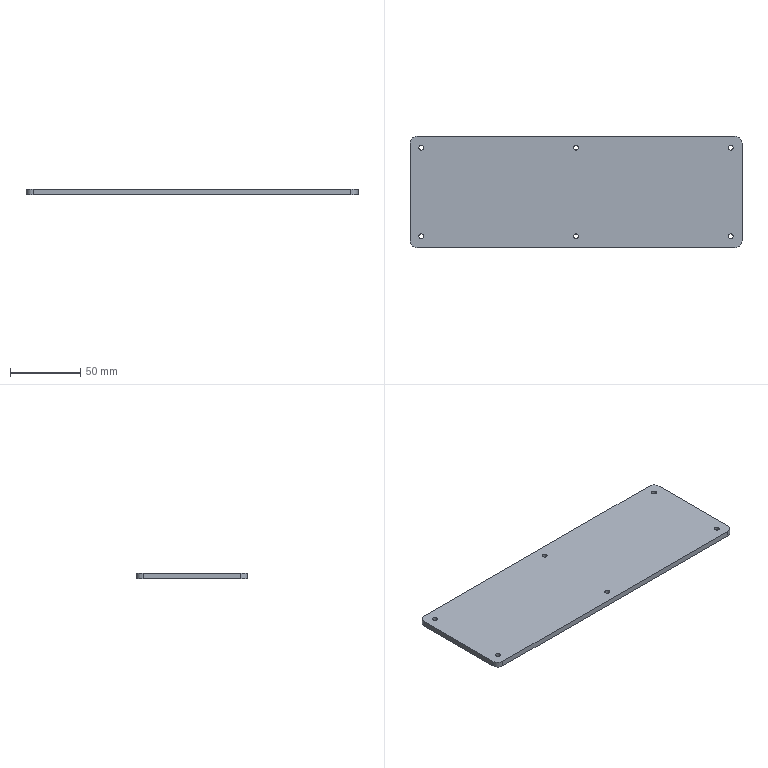Part | SolidWorks | features Extrusion 1, Fillet 1, ICE 1 | 1 solid | 22 faces | box 236 x 79 x 4 mm | volume 74259 mm3 | cylinder 16 | plane 6 | commonest cylinder face diameters 3.5 x12 10 x4
STEP:
#1=CARTESIAN_POINT('',(-108.25,31.5,4.));
#2=VERTEX_POINT('',#1);
#3=CARTESIAN_POINT('',(-111.75,31.5,4.));
#4=VERTEX_POINT('',#3);
#5=CARTESIAN_POINT('',(-110.,31.5,4.));
#6=DIRECTION('',(0.,0.,-1.));
#7=DIRECTION('',(-1.,0.,0.));
#8=AXIS2_PLACEMENT_3D('',#5,#6,#7);
#9=CIRCLE('',#8,1.75);
#10=EDGE_CURVE('',#2,#4,#9,.T.);
#11=ORIENTED_EDGE('',*,*,#10,.F.);
#12=CARTESIAN_POINT('',(-108.25,31.5,0.));
#13=VERTEX_POINT('',#12);
#14=CARTESIAN_POINT('',(-108.25,31.5,4.));
#15=DIRECTION('',(0.,0.,-1.));
#16=VECTOR('',#15,1000.);
#17=LINE('',#14,#16);
#18=EDGE_CURVE('',#2,#13,#17,.T.);
#19=ORIENTED_EDGE('',*,*,#18,.T.);
#20=CARTESIAN_POINT('',(-111.75,31.5,0.));
#21=VERTEX_POINT('',#20);
#22=CARTESIAN_POINT('',(-110.,31.5,0.));
#23=DIRECTION('',(0.,0.,-1.));
#24=DIRECTION('',(-1.,0.,0.));
#25=AXIS2_PLACEMENT_3D('',#22,#23,#24);
#26=CIRCLE('',#25,1.75);
#27=EDGE_CURVE('',#13,#21,#26,.T.);
#28=ORIENTED_EDGE('',*,*,#27,.T.);
#29=CARTESIAN_POINT('',(-111.75,31.5,4.));
#30=DIRECTION('',(0.,0.,-1.));
#31=VECTOR('',#30,1000.);
#32=LINE('',#29,#31);
#33=EDGE_CURVE('',#4,#21,#32,.T.);
#34=ORIENTED_EDGE('',*,*,#33,.F.);
#35=EDGE_LOOP('',(#11,#19,#28,#34));
#36=FACE_OUTER_BOUND('',#35,.T.);
#37=CARTESIAN_POINT('',(-110.,31.5,4.));
#38=DIRECTION('',(0.,0.,-1.));
#39=DIRECTION('',(-1.,0.,0.));
#40=AXIS2_PLACEMENT_3D('',#37,#38,#39);
#41=CYLINDRICAL_SURFACE('',#40,1.75);
#42=ADVANCED_FACE('',(#36),#41,.F.);
#43=CARTESIAN_POINT('',(-108.25,-31.5,4.));
#44=VERTEX_POINT('',#43);
#45=CARTESIAN_POINT('',(-111.75,-31.5,4.));
#46=VERTEX_POINT('',#45);
#47=CARTESIAN_POINT('',(-110.,-31.5,4.));
#48=DIRECTION('',(0.,0.,-1.));
#49=DIRECTION('',(-1.,0.,0.));
#50=AXIS2_PLACEMENT_3D('',#47,#48,#49);
#51=CIRCLE('',#50,1.75);
#52=EDGE_CURVE('',#44,#46,#51,.T.);
#53=ORIENTED_EDGE('',*,*,#52,.F.);
#54=CARTESIAN_POINT('',(-108.25,-31.5,0.));
#55=VERTEX_POINT('',#54);
#56=CARTESIAN_POINT('',(-108.25,-31.5,4.));
#57=DIRECTION('',(0.,0.,-1.));
#58=VECTOR('',#57,1000.);
#59=LINE('',#56,#58);
#60=EDGE_CURVE('',#44,#55,#59,.T.);
#61=ORIENTED_EDGE('',*,*,#60,.T.);
#62=CARTESIAN_POINT('',(-111.75,-31.5,0.));
#63=VERTEX_POINT('',#62);
#64=CARTESIAN_POINT('',(-110.,-31.5,0.));
#65=DIRECTION('',(0.,0.,-1.));
#66=DIRECTION('',(-1.,0.,0.));
#67=AXIS2_PLACEMENT_3D('',#64,#65,#66);
#68=CIRCLE('',#67,1.75);
#69=EDGE_CURVE('',#55,#63,#68,.T.);
#70=ORIENTED_EDGE('',*,*,#69,.T.);
#71=CARTESIAN_POINT('',(-111.75,-31.5,4.));
#72=DIRECTION('',(0.,0.,-1.));
#73=VECTOR('',#72,1000.);
#74=LINE('',#71,#73);
#75=EDGE_CURVE('',#46,#63,#74,.T.);
#76=ORIENTED_EDGE('',*,*,#75,.F.);
#77=EDGE_LOOP('',(#53,#61,#70,#76));
#78=FACE_OUTER_BOUND('',#77,.T.);
#79=CARTESIAN_POINT('',(-110.,-31.5,4.));
#80=DIRECTION('',(0.,0.,-1.));
#81=DIRECTION('',(-1.,0.,0.));
#82=AXIS2_PLACEMENT_3D('',#79,#80,#81);
#83=CYLINDRICAL_SURFACE('',#82,1.75);
#84=ADVANCED_FACE('',(#78),#83,.F.);
#85=CARTESIAN_POINT('',(111.75,-31.5,4.));
#86=VERTEX_POINT('',#85);
#87=CARTESIAN_POINT('',(108.25,-31.5,4.));
#88=VERTEX_POINT('',#87);
#89=CARTESIAN_POINT('',(110.,-31.5,4.));
#90=DIRECTION('',(0.,0.,-1.));
#91=DIRECTION('',(-1.,0.,0.));
#92=AXIS2_PLACEMENT_3D('',#89,#90,#91);
#93=CIRCLE('',#92,1.75);
#94=EDGE_CURVE('',#86,#88,#93,.T.);
#95=ORIENTED_EDGE('',*,*,#94,.F.);
#96=CARTESIAN_POINT('',(111.75,-31.5,0.));
#97=VERTEX_POINT('',#96);
#98=CARTESIAN_POINT('',(111.75,-31.5,4.));
#99=DIRECTION('',(0.,0.,-1.));
#100=VECTOR('',#99,1000.);
#101=LINE('',#98,#100);
#102=EDGE_CURVE('',#86,#97,#101,.T.);
#103=ORIENTED_EDGE('',*,*,#102,.T.);
#104=CARTESIAN_POINT('',(108.25,-31.5,0.));
#105=VERTEX_POINT('',#104);
#106=CARTESIAN_POINT('',(110.,-31.5,0.));
#107=DIRECTION('',(0.,0.,-1.));
#108=DIRECTION('',(-1.,0.,0.));
#109=AXIS2_PLACEMENT_3D('',#106,#107,#108);
#110=CIRCLE('',#109,1.75);
#111=EDGE_CURVE('',#97,#105,#110,.T.);
#112=ORIENTED_EDGE('',*,*,#111,.T.);
#113=CARTESIAN_POINT('',(108.25,-31.5,4.));
#114=DIRECTION('',(0.,0.,-1.));
#115=VECTOR('',#114,1000.);
#116=LINE('',#113,#115);
#117=EDGE_CURVE('',#88,#105,#116,.T.);
#118=ORIENTED_EDGE('',*,*,#117,.F.);
#119=EDGE_LOOP('',(#95,#103,#112,#118));
#120=FACE_OUTER_BOUND('',#119,.T.);
#121=CARTESIAN_POINT('',(110.,-31.5,4.));
#122=DIRECTION('',(0.,0.,-1.));
#123=DIRECTION('',(-1.,0.,0.));
#124=AXIS2_PLACEMENT_3D('',#121,#122,#123);
#125=CYLINDRICAL_SURFACE('',#124,1.75);
#126=ADVANCED_FACE('',(#120),#125,.F.);
#127=CARTESIAN_POINT('',(1.75,31.5,4.));
#128=VERTEX_POINT('',#127);
#129=CARTESIAN_POINT('',(-1.75,31.5,4.));
#130=VERTEX_POINT('',#129);
#131=CARTESIAN_POINT('',(0.,31.5,4.));
#132=DIRECTION('',(0.,0.,-1.));
#133=DIRECTION('',(-1.,0.,0.));
#134=AXIS2_PLACEMENT_3D('',#131,#132,#133);
#135=CIRCLE('',#134,1.75);
#136=EDGE_CURVE('',#128,#130,#135,.T.);
#137=ORIENTED_EDGE('',*,*,#136,.F.);
#138=CARTESIAN_POINT('',(1.75,31.5,0.));
#139=VERTEX_POINT('',#138);
#140=CARTESIAN_POINT('',(1.75,31.5,4.));
#141=DIRECTION('',(0.,0.,-1.));
#142=VECTOR('',#141,1000.);
#143=LINE('',#140,#142);
#144=EDGE_CURVE('',#128,#139,#143,.T.);
#145=ORIENTED_EDGE('',*,*,#144,.T.);
#146=CARTESIAN_POINT('',(-1.75,31.5,0.));
#147=VERTEX_POINT('',#146);
#148=CARTESIAN_POINT('',(0.,31.5,0.));
#149=DIRECTION('',(0.,0.,-1.));
#150=DIRECTION('',(-1.,0.,0.));
#151=AXIS2_PLACEMENT_3D('',#148,#149,#150);
#152=CIRCLE('',#151,1.75);
#153=EDGE_CURVE('',#139,#147,#152,.T.);
#154=ORIENTED_EDGE('',*,*,#153,.T.);
#155=CARTESIAN_POINT('',(-1.75,31.5,4.));
#156=DIRECTION('',(0.,0.,-1.));
#157=VECTOR('',#156,1000.);
#158=LINE('',#155,#157);
#159=EDGE_CURVE('',#130,#147,#158,.T.);
#160=ORIENTED_EDGE('',*,*,#159,.F.);
#161=EDGE_LOOP('',(#137,#145,#154,#160));
#162=FACE_OUTER_BOUND('',#161,.T.);
#163=CARTESIAN_POINT('',(0.,31.5,4.));
#164=DIRECTION('',(0.,0.,-1.));
#165=DIRECTION('',(-1.,0.,0.));
#166=AXIS2_PLACEMENT_3D('',#163,#164,#165);
#167=CYLINDRICAL_SURFACE('',#166,1.75);
#168=ADVANCED_FACE('',(#162),#167,.F.);
#169=CARTESIAN_POINT('',(1.75,-31.5,4.));
#170=VERTEX_POINT('',#169);
#171=CARTESIAN_POINT('',(-1.75,-31.5,4.));
#172=VERTEX_POINT('',#171);
#173=CARTESIAN_POINT('',(0.,-31.5,4.));
#174=DIRECTION('',(0.,0.,-1.));
#175=DIRECTION('',(-1.,0.,0.));
#176=AXIS2_PLACEMENT_3D('',#173,#174,#175);
#177=CIRCLE('',#176,1.75);
#178=EDGE_CURVE('',#170,#172,#177,.T.);
#179=ORIENTED_EDGE('',*,*,#178,.F.);
#180=CARTESIAN_POINT('',(1.75,-31.5,0.));
#181=VERTEX_POINT('',#180);
#182=CARTESIAN_POINT('',(1.75,-31.5,4.));
#183=DIRECTION('',(0.,0.,-1.));
#184=VECTOR('',#183,1000.);
#185=LINE('',#182,#184);
#186=EDGE_CURVE('',#170,#181,#185,.T.);
#187=ORIENTED_EDGE('',*,*,#186,.T.);
#188=CARTESIAN_POINT('',(-1.75,-31.5,0.));
#189=VERTEX_POINT('',#188);
#190=CARTESIAN_POINT('',(0.,-31.5,0.));
#191=DIRECTION('',(0.,0.,-1.));
#192=DIRECTION('',(-1.,0.,0.));
#193=AXIS2_PLACEMENT_3D('',#190,#191,#192);
#194=CIRCLE('',#193,1.75);
#195=EDGE_CURVE('',#181,#189,#194,.T.);
#196=ORIENTED_EDGE('',*,*,#195,.T.);
#197=CARTESIAN_POINT('',(-1.75,-31.5,4.));
#198=DIRECTION('',(0.,0.,-1.));
#199=VECTOR('',#198,1000.);
#200=LINE('',#197,#199);
#201=EDGE_CURVE('',#172,#189,#200,.T.);
#202=ORIENTED_EDGE('',*,*,#201,.F.);
#203=EDGE_LOOP('',(#179,#187,#196,#202));
#204=FACE_OUTER_BOUND('',#203,.T.);
#205=CARTESIAN_POINT('',(0.,-31.5,4.));
#206=DIRECTION('',(0.,0.,-1.));
#207=DIRECTION('',(-1.,0.,0.));
#208=AXIS2_PLACEMENT_3D('',#205,#206,#207);
#209=CYLINDRICAL_SURFACE('',#208,1.75);
#210=ADVANCED_FACE('',(#204),#209,.F.);
#211=CARTESIAN_POINT('',(111.75,31.5,4.));
#212=VERTEX_POINT('',#211);
#213=CARTESIAN_POINT('',(108.25,31.5,4.));
#214=VERTEX_POINT('',#213);
#215=CARTESIAN_POINT('',(110.,31.5,4.));
#216=DIRECTION('',(0.,0.,-1.));
#217=DIRECTION('',(-1.,0.,0.));
#218=AXIS2_PLACEMENT_3D('',#215,#216,#217);
#219=CIRCLE('',#218,1.75);
#220=EDGE_CURVE('',#212,#214,#219,.T.);
#221=ORIENTED_EDGE('',*,*,#220,.F.);
#222=CARTESIAN_POINT('',(111.75,31.5,0.));
#223=VERTEX_POINT('',#222);
#224=CARTESIAN_POINT('',(111.75,31.5,4.));
#225=DIRECTION('',(0.,0.,-1.));
#226=VECTOR('',#225,1000.);
#227=LINE('',#224,#226);
#228=EDGE_CURVE('',#212,#223,#227,.T.);
#229=ORIENTED_EDGE('',*,*,#228,.T.);
#230=CARTESIAN_POINT('',(108.25,31.5,0.));
#231=VERTEX_POINT('',#230);
#232=CARTESIAN_POINT('',(110.,31.5,0.));
#233=DIRECTION('',(0.,0.,-1.));
#234=DIRECTION('',(-1.,0.,0.));
#235=AXIS2_PLACEMENT_3D('',#232,#233,#234);
#236=CIRCLE('',#235,1.75);
#237=EDGE_CURVE('',#223,#231,#236,.T.);
#238=ORIENTED_EDGE('',*,*,#237,.T.);
#239=CARTESIAN_POINT('',(108.25,31.5,4.));
#240=DIRECTION('',(0.,0.,-1.));
#241=VECTOR('',#240,1000.);
#242=LINE('',#239,#241);
#243=EDGE_CURVE('',#214,#231,#242,.T.);
#244=ORIENTED_EDGE('',*,*,#243,.F.);
#245=EDGE_LOOP('',(#221,#229,#238,#244));
#246=FACE_OUTER_BOUND('',#245,.T.);
#247=CARTESIAN_POINT('',(110.,31.5,4.));
#248=DIRECTION('',(0.,0.,-1.));
#249=DIRECTION('',(-1.,0.,0.));
#250=AXIS2_PLACEMENT_3D('',#247,#248,#249);
#251=CYLINDRICAL_SURFACE('',#250,1.75);
#252=ADVANCED_FACE('',(#246),#251,.F.);
#253=CARTESIAN_POINT('',(-118.,34.5,0.));
#254=VERTEX_POINT('',#253);
#255=CARTESIAN_POINT('',(-118.,-34.5,0.));
#256=VERTEX_POINT('',#255);
#257=CARTESIAN_POINT('',(-118.,-39.5,0.));
#258=DIRECTION('',(0.,-1.,0.));
#259=VECTOR('',#258,1000.);
#260=LINE('',#257,#259);
#261=EDGE_CURVE('',#254,#256,#260,.T.);
#262=ORIENTED_EDGE('',*,*,#261,.T.);
#263=CARTESIAN_POINT('',(-118.,-34.5,4.));
#264=VERTEX_POINT('',#263);
#265=CARTESIAN_POINT('',(-118.,-34.5,4.));
#266=DIRECTION('',(0.,0.,1.));
#267=VECTOR('',#266,1000.);
#268=LINE('',#265,#267);
#269=EDGE_CURVE('',#256,#264,#268,.T.);
#270=ORIENTED_EDGE('',*,*,#269,.T.);
#271=CARTESIAN_POINT('',(-118.,34.5,4.));
#272=VERTEX_POINT('',#271);
#273=CARTESIAN_POINT('',(-118.,-39.5,4.));
#274=DIRECTION('',(0.,-1.,0.));
#275=VECTOR('',#274,1000.);
#276=LINE('',#273,#275);
#277=EDGE_CURVE('',#272,#264,#276,.T.);
#278=ORIENTED_EDGE('',*,*,#277,.F.);
#279=CARTESIAN_POINT('',(-118.,34.5,4.));
#280=DIRECTION('',(0.,0.,-1.));
#281=VECTOR('',#280,1000.);
#282=LINE('',#279,#281);
#283=EDGE_CURVE('',#272,#254,#282,.T.);
#284=ORIENTED_EDGE('',*,*,#283,.T.);
#285=EDGE_LOOP('',(#262,#270,#278,#284));
#286=FACE_OUTER_BOUND('',#285,.T.);
#287=CARTESIAN_POINT('',(-118.,-39.5,4.));
#288=DIRECTION('',(1.,0.,0.));
#289=DIRECTION('',(0.,0.,-1.));
#290=AXIS2_PLACEMENT_3D('',#287,#288,#289);
#291=PLANE('',#290);
#292=ADVANCED_FACE('',(#286),#291,.F.);
#293=CARTESIAN_POINT('',(-113.,-39.5,0.));
#294=VERTEX_POINT('',#293);
#295=CARTESIAN_POINT('',(113.,-39.5,0.));
#296=VERTEX_POINT('',#295);
#297=CARTESIAN_POINT('',(118.,-39.5,0.));
#298=DIRECTION('',(1.,0.,0.));
#299=VECTOR('',#298,1000.);
#300=LINE('',#297,#299);
#301=EDGE_CURVE('',#294,#296,#300,.T.);
#302=ORIENTED_EDGE('',*,*,#301,.T.);
#303=CARTESIAN_POINT('',(113.,-39.5,4.));
#304=VERTEX_POINT('',#303);
#305=CARTESIAN_POINT('',(113.,-39.5,4.));
#306=DIRECTION('',(0.,0.,1.));
#307=VECTOR('',#306,1000.);
#308=LINE('',#305,#307);
#309=EDGE_CURVE('',#296,#304,#308,.T.);
#310=ORIENTED_EDGE('',*,*,#309,.T.);
#311=CARTESIAN_POINT('',(-113.,-39.5,4.));
#312=VERTEX_POINT('',#311);
#313=CARTESIAN_POINT('',(118.,-39.5,4.));
#314=DIRECTION('',(1.,0.,0.));
#315=VECTOR('',#314,1000.);
#316=LINE('',#313,#315);
#317=EDGE_CURVE('',#312,#304,#316,.T.);
#318=ORIENTED_EDGE('',*,*,#317,.F.);
#319=CARTESIAN_POINT('',(-113.,-39.5,4.));
#320=DIRECTION('',(0.,0.,-1.));
#321=VECTOR('',#320,1000.);
#322=LINE('',#319,#321);
#323=EDGE_CURVE('',#312,#294,#322,.T.);
#324=ORIENTED_EDGE('',*,*,#323,.T.);
#325=EDGE_LOOP('',(#302,#310,#318,#324));
#326=FACE_OUTER_BOUND('',#325,.T.);
#327=CARTESIAN_POINT('',(118.,-39.5,4.));
#328=DIRECTION('',(0.,1.,0.));
#329=DIRECTION('',(-1.,0.,0.));
#330=AXIS2_PLACEMENT_3D('',#327,#328,#329);
#331=PLANE('',#330);
#332=ADVANCED_FACE('',(#326),#331,.F.);
#333=CARTESIAN_POINT('',(118.,-34.5,0.));
#334=VERTEX_POINT('',#333);
#335=CARTESIAN_POINT('',(118.,34.5,0.));
#336=VERTEX_POINT('',#335);
#337=CARTESIAN_POINT('',(118.,-39.5,0.));
#338=DIRECTION('',(0.,1.,0.));
#339=VECTOR('',#338,1000.);
#340=LINE('',#337,#339);
#341=EDGE_CURVE('',#334,#336,#340,.T.);
#342=ORIENTED_EDGE('',*,*,#341,.T.);
#343=CARTESIAN_POINT('',(118.,34.5,4.));
#344=VERTEX_POINT('',#343);
#345=CARTESIAN_POINT('',(118.,34.5,4.));
#346=DIRECTION('',(0.,0.,1.));
#347=VECTOR('',#346,1000.);
#348=LINE('',#345,#347);
#349=EDGE_CURVE('',#336,#344,#348,.T.);
#350=ORIENTED_EDGE('',*,*,#349,.T.);
#351=CARTESIAN_POINT('',(118.,-34.5,4.));
#352=VERTEX_POINT('',#351);
#353=CARTESIAN_POINT('',(118.,-39.5,4.));
#354=DIRECTION('',(0.,1.,0.));
#355=VECTOR('',#354,1000.);
#356=LINE('',#353,#355);
#357=EDGE_CURVE('',#352,#344,#356,.T.);
#358=ORIENTED_EDGE('',*,*,#357,.F.);
#359=CARTESIAN_POINT('',(118.,-34.5,4.));
#360=DIRECTION('',(0.,0.,-1.));
#361=VECTOR('',#360,1000.);
#362=LINE('',#359,#361);
#363=EDGE_CURVE('',#352,#334,#362,.T.);
#364=ORIENTED_EDGE('',*,*,#363,.T.);
#365=EDGE_LOOP('',(#342,#350,#358,#364));
#366=FACE_OUTER_BOUND('',#365,.T.);
#367=CARTESIAN_POINT('',(118.,-39.5,4.));
#368=DIRECTION('',(-1.,0.,0.));
#369=DIRECTION('',(0.,0.,1.));
#370=AXIS2_PLACEMENT_3D('',#367,#368,#369);
#371=PLANE('',#370);
#372=ADVANCED_FACE('',(#366),#371,.F.);
#373=CARTESIAN_POINT('',(113.,39.5,4.));
#374=VERTEX_POINT('',#373);
#375=CARTESIAN_POINT('',(-113.,39.5,4.));
#376=VERTEX_POINT('',#375);
#377=CARTESIAN_POINT('',(118.,39.5,4.));
#378=DIRECTION('',(-1.,0.,0.));
#379=VECTOR('',#378,1000.);
#380=LINE('',#377,#379);
#381=EDGE_CURVE('',#374,#376,#380,.T.);
#382=ORIENTED_EDGE('',*,*,#381,.F.);
#383=CARTESIAN_POINT('',(113.,39.5,0.));
#384=VERTEX_POINT('',#383);
#385=CARTESIAN_POINT('',(113.,39.5,4.));
#386=DIRECTION('',(0.,0.,-1.));
#387=VECTOR('',#386,1000.);
#388=LINE('',#385,#387);
#389=EDGE_CURVE('',#374,#384,#388,.T.);
#390=ORIENTED_EDGE('',*,*,#389,.T.);
#391=CARTESIAN_POINT('',(-113.,39.5,0.));
#392=VERTEX_POINT('',#391);
#393=CARTESIAN_POINT('',(118.,39.5,0.));
#394=DIRECTION('',(-1.,0.,0.));
#395=VECTOR('',#394,1000.);
#396=LINE('',#393,#395);
#397=EDGE_CURVE('',#384,#392,#396,.T.);
#398=ORIENTED_EDGE('',*,*,#397,.T.);
#399=CARTESIAN_POINT('',(-113.,39.5,4.));
#400=DIRECTION('',(0.,0.,1.));
#401=VECTOR('',#400,1000.);
#402=LINE('',#399,#401);
#403=EDGE_CURVE('',#392,#376,#402,.T.);
#404=ORIENTED_EDGE('',*,*,#403,.T.);
#405=EDGE_LOOP('',(#382,#390,#398,#404));
#406=FACE_OUTER_BOUND('',#405,.T.);
#407=CARTESIAN_POINT('',(118.,39.5,4.));
#408=DIRECTION('',(0.,-1.,0.));
#409=DIRECTION('',(1.,0.,0.));
#410=AXIS2_PLACEMENT_3D('',#407,#408,#409);
#411=PLANE('',#410);
#412=ADVANCED_FACE('',(#406),#411,.F.);
#413=CARTESIAN_POINT('',(-110.,31.5,4.));
#414=DIRECTION('',(0.,0.,-1.));
#415=DIRECTION('',(-1.,0.,0.));
#416=AXIS2_PLACEMENT_3D('',#413,#414,#415);
#417=CIRCLE('',#416,1.75);
#418=EDGE_CURVE('',#4,#2,#417,.T.);
#419=ORIENTED_EDGE('',*,*,#418,.T.);
#420=ORIENTED_EDGE('',*,*,#10,.T.);
#421=EDGE_LOOP('',(#419,#420));
#422=FACE_BOUND('',#421,.T.);
#423=CARTESIAN_POINT('',(-110.,-31.5,4.));
#424=DIRECTION('',(0.,0.,-1.));
#425=DIRECTION('',(-1.,0.,0.));
#426=AXIS2_PLACEMENT_3D('',#423,#424,#425);
#427=CIRCLE('',#426,1.75);
#428=EDGE_CURVE('',#46,#44,#427,.T.);
#429=ORIENTED_EDGE('',*,*,#428,.T.);
#430=ORIENTED_EDGE('',*,*,#52,.T.);
#431=EDGE_LOOP('',(#429,#430));
#432=FACE_BOUND('',#431,.T.);
#433=CARTESIAN_POINT('',(110.,-31.5,4.));
#434=DIRECTION('',(0.,0.,-1.));
#435=DIRECTION('',(-1.,0.,0.));
#436=AXIS2_PLACEMENT_3D('',#433,#434,#435);
#437=CIRCLE('',#436,1.75);
#438=EDGE_CURVE('',#88,#86,#437,.T.);
#439=ORIENTED_EDGE('',*,*,#438,.T.);
#440=ORIENTED_EDGE('',*,*,#94,.T.);
#441=EDGE_LOOP('',(#439,#440));
#442=FACE_BOUND('',#441,.T.);
#443=CARTESIAN_POINT('',(0.,31.5,4.));
#444=DIRECTION('',(0.,0.,-1.));
#445=DIRECTION('',(-1.,0.,0.));
#446=AXIS2_PLACEMENT_3D('',#443,#444,#445);
#447=CIRCLE('',#446,1.75);
#448=EDGE_CURVE('',#130,#128,#447,.T.);
#449=ORIENTED_EDGE('',*,*,#448,.T.);
#450=ORIENTED_EDGE('',*,*,#136,.T.);
#451=EDGE_LOOP('',(#449,#450));
#452=FACE_BOUND('',#451,.T.);
#453=CARTESIAN_POINT('',(0.,-31.5,4.));
#454=DIRECTION('',(0.,0.,-1.));
#455=DIRECTION('',(-1.,0.,0.));
#456=AXIS2_PLACEMENT_3D('',#453,#454,#455);
#457=CIRCLE('',#456,1.75);
#458=EDGE_CURVE('',#172,#170,#457,.T.);
#459=ORIENTED_EDGE('',*,*,#458,.T.);
#460=ORIENTED_EDGE('',*,*,#178,.T.);
#461=EDGE_LOOP('',(#459,#460));
#462=FACE_BOUND('',#461,.T.);
#463=CARTESIAN_POINT('',(110.,31.5,4.));
#464=DIRECTION('',(0.,0.,-1.));
#465=DIRECTION('',(-1.,0.,0.));
#466=AXIS2_PLACEMENT_3D('',#463,#464,#465);
#467=CIRCLE('',#466,1.75);
#468=EDGE_CURVE('',#214,#212,#467,.T.);
#469=ORIENTED_EDGE('',*,*,#468,.T.);
#470=ORIENTED_EDGE('',*,*,#220,.T.);
#471=EDGE_LOOP('',(#469,#470));
#472=FACE_BOUND('',#471,.T.);
#473=ORIENTED_EDGE('',*,*,#357,.T.);
#474=CARTESIAN_POINT('',(113.,34.5,4.));
#475=DIRECTION('',(0.,0.,1.));
#476=DIRECTION('',(1.,0.,0.));
#477=AXIS2_PLACEMENT_3D('',#474,#475,#476);
#478=CIRCLE('',#477,5.);
#479=EDGE_CURVE('',#344,#374,#478,.T.);
#480=ORIENTED_EDGE('',*,*,#479,.T.);
#481=ORIENTED_EDGE('',*,*,#381,.T.);
#482=CARTESIAN_POINT('',(-113.,34.5,4.));
#483=DIRECTION('',(0.,0.,1.));
#484=DIRECTION('',(1.,0.,0.));
#485=AXIS2_PLACEMENT_3D('',#482,#483,#484);
#486=CIRCLE('',#485,5.);
#487=EDGE_CURVE('',#376,#272,#486,.T.);
#488=ORIENTED_EDGE('',*,*,#487,.T.);
#489=ORIENTED_EDGE('',*,*,#277,.T.);
#490=CARTESIAN_POINT('',(-113.,-34.5,4.));
#491=DIRECTION('',(0.,0.,1.));
#492=DIRECTION('',(1.,0.,0.));
#493=AXIS2_PLACEMENT_3D('',#490,#491,#492);
#494=CIRCLE('',#493,5.);
#495=EDGE_CURVE('',#264,#312,#494,.T.);
#496=ORIENTED_EDGE('',*,*,#495,.T.);
#497=ORIENTED_EDGE('',*,*,#317,.T.);
#498=CARTESIAN_POINT('',(113.,-34.5,4.));
#499=DIRECTION('',(0.,0.,1.));
#500=DIRECTION('',(1.,0.,0.));
#501=AXIS2_PLACEMENT_3D('',#498,#499,#500);
#502=CIRCLE('',#501,5.);
#503=EDGE_CURVE('',#304,#352,#502,.T.);
#504=ORIENTED_EDGE('',*,*,#503,.T.);
#505=EDGE_LOOP('',(#473,#480,#481,#488,#489,#496,#497,#504));
#506=FACE_OUTER_BOUND('',#505,.T.);
#507=CARTESIAN_POINT('',(0.,0.,4.));
#508=DIRECTION('',(0.,0.,1.));
#509=DIRECTION('',(1.,0.,0.));
#510=AXIS2_PLACEMENT_3D('',#507,#508,#509);
#511=PLANE('',#510);
#512=ADVANCED_FACE('',(#422,#432,#442,#452,#462,#472,#506),#511,.T.);
#513=CARTESIAN_POINT('',(-110.,31.5,0.));
#514=DIRECTION('',(0.,0.,-1.));
#515=DIRECTION('',(-1.,0.,0.));
#516=AXIS2_PLACEMENT_3D('',#513,#514,#515);
#517=CIRCLE('',#516,1.75);
#518=EDGE_CURVE('',#21,#13,#517,.T.);
#519=ORIENTED_EDGE('',*,*,#518,.F.);
#520=ORIENTED_EDGE('',*,*,#27,.F.);
#521=EDGE_LOOP('',(#519,#520));
#522=FACE_BOUND('',#521,.T.);
#523=CARTESIAN_POINT('',(-110.,-31.5,0.));
#524=DIRECTION('',(0.,0.,-1.));
#525=DIRECTION('',(-1.,0.,0.));
#526=AXIS2_PLACEMENT_3D('',#523,#524,#525);
#527=CIRCLE('',#526,1.75);
#528=EDGE_CURVE('',#63,#55,#527,.T.);
#529=ORIENTED_EDGE('',*,*,#528,.F.);
#530=ORIENTED_EDGE('',*,*,#69,.F.);
#531=EDGE_LOOP('',(#529,#530));
#532=FACE_BOUND('',#531,.T.);
#533=CARTESIAN_POINT('',(110.,-31.5,0.));
#534=DIRECTION('',(0.,0.,-1.));
#535=DIRECTION('',(-1.,0.,0.));
#536=AXIS2_PLACEMENT_3D('',#533,#534,#535);
#537=CIRCLE('',#536,1.75);
#538=EDGE_CURVE('',#105,#97,#537,.T.);
#539=ORIENTED_EDGE('',*,*,#538,.F.);
#540=ORIENTED_EDGE('',*,*,#111,.F.);
#541=EDGE_LOOP('',(#539,#540));
#542=FACE_BOUND('',#541,.T.);
#543=CARTESIAN_POINT('',(0.,31.5,0.));
#544=DIRECTION('',(0.,0.,-1.));
#545=DIRECTION('',(-1.,0.,0.));
#546=AXIS2_PLACEMENT_3D('',#543,#544,#545);
#547=CIRCLE('',#546,1.75);
#548=EDGE_CURVE('',#147,#139,#547,.T.);
#549=ORIENTED_EDGE('',*,*,#548,.F.);
#550=ORIENTED_EDGE('',*,*,#153,.F.);
#551=EDGE_LOOP('',(#549,#550));
#552=FACE_BOUND('',#551,.T.);
#553=CARTESIAN_POINT('',(0.,-31.5,0.));
#554=DIRECTION('',(0.,0.,-1.));
#555=DIRECTION('',(-1.,0.,0.));
#556=AXIS2_PLACEMENT_3D('',#553,#554,#555);
#557=CIRCLE('',#556,1.75);
#558=EDGE_CURVE('',#189,#181,#557,.T.);
#559=ORIENTED_EDGE('',*,*,#558,.F.);
#560=ORIENTED_EDGE('',*,*,#195,.F.);
#561=EDGE_LOOP('',(#559,#560));
#562=FACE_BOUND('',#561,.T.);
#563=CARTESIAN_POINT('',(110.,31.5,0.));
#564=DIRECTION('',(0.,0.,-1.));
#565=DIRECTION('',(-1.,0.,0.));
#566=AXIS2_PLACEMENT_3D('',#563,#564,#565);
#567=CIRCLE('',#566,1.75);
#568=EDGE_CURVE('',#231,#223,#567,.T.);
#569=ORIENTED_EDGE('',*,*,#568,.F.);
#570=ORIENTED_EDGE('',*,*,#237,.F.);
#571=EDGE_LOOP('',(#569,#570));
#572=FACE_BOUND('',#571,.T.);
#573=ORIENTED_EDGE('',*,*,#397,.F.);
#574=CARTESIAN_POINT('',(113.,34.5,0.));
#575=DIRECTION('',(0.,0.,-1.));
#576=DIRECTION('',(1.,0.,0.));
#577=AXIS2_PLACEMENT_3D('',#574,#575,#576);
#578=CIRCLE('',#577,5.);
#579=EDGE_CURVE('',#384,#336,#578,.T.);
#580=ORIENTED_EDGE('',*,*,#579,.T.);
#581=ORIENTED_EDGE('',*,*,#341,.F.);
#582=CARTESIAN_POINT('',(113.,-34.5,0.));
#583=DIRECTION('',(0.,0.,-1.));
#584=DIRECTION('',(1.,0.,0.));
#585=AXIS2_PLACEMENT_3D('',#582,#583,#584);
#586=CIRCLE('',#585,5.);
#587=EDGE_CURVE('',#334,#296,#586,.T.);
#588=ORIENTED_EDGE('',*,*,#587,.T.);
#589=ORIENTED_EDGE('',*,*,#301,.F.);
#590=CARTESIAN_POINT('',(-113.,-34.5,0.));
#591=DIRECTION('',(0.,0.,-1.));
#592=DIRECTION('',(1.,0.,0.));
#593=AXIS2_PLACEMENT_3D('',#590,#591,#592);
#594=CIRCLE('',#593,5.);
#595=EDGE_CURVE('',#294,#256,#594,.T.);
#596=ORIENTED_EDGE('',*,*,#595,.T.);
#597=ORIENTED_EDGE('',*,*,#261,.F.);
#598=CARTESIAN_POINT('',(-113.,34.5,0.));
#599=DIRECTION('',(0.,0.,-1.));
#600=DIRECTION('',(1.,0.,0.));
#601=AXIS2_PLACEMENT_3D('',#598,#599,#600);
#602=CIRCLE('',#601,5.);
#603=EDGE_CURVE('',#254,#392,#602,.T.);
#604=ORIENTED_EDGE('',*,*,#603,.T.);
#605=EDGE_LOOP('',(#573,#580,#581,#588,#589,#596,#597,#604));
#606=FACE_OUTER_BOUND('',#605,.T.);
#607=CARTESIAN_POINT('',(0.,0.,0.));
#608=DIRECTION('',(0.,0.,1.));
#609=DIRECTION('',(1.,0.,0.));
#610=AXIS2_PLACEMENT_3D('',#607,#608,#609);
#611=PLANE('',#610);
#612=ADVANCED_FACE('',(#522,#532,#542,#552,#562,#572,#606),#611,.F.);
#613=ORIENTED_EDGE('',*,*,#479,.F.);
#614=ORIENTED_EDGE('',*,*,#349,.F.);
#615=ORIENTED_EDGE('',*,*,#579,.F.);
#616=ORIENTED_EDGE('',*,*,#389,.F.);
#617=EDGE_LOOP('',(#613,#614,#615,#616));
#618=FACE_OUTER_BOUND('',#617,.T.);
#619=CARTESIAN_POINT('',(113.,34.5,4.));
#620=DIRECTION('',(0.,0.,-1.));
#621=DIRECTION('',(-1.,0.,0.));
#622=AXIS2_PLACEMENT_3D('',#619,#620,#621);
#623=CYLINDRICAL_SURFACE('',#622,5.);
#624=ADVANCED_FACE('',(#618),#623,.T.);
#625=ORIENTED_EDGE('',*,*,#503,.F.);
#626=ORIENTED_EDGE('',*,*,#309,.F.);
#627=ORIENTED_EDGE('',*,*,#587,.F.);
#628=ORIENTED_EDGE('',*,*,#363,.F.);
#629=EDGE_LOOP('',(#625,#626,#627,#628));
#630=FACE_OUTER_BOUND('',#629,.T.);
#631=CARTESIAN_POINT('',(113.,-34.5,4.));
#632=DIRECTION('',(0.,0.,-1.));
#633=DIRECTION('',(-1.,0.,0.));
#634=AXIS2_PLACEMENT_3D('',#631,#632,#633);
#635=CYLINDRICAL_SURFACE('',#634,5.);
#636=ADVANCED_FACE('',(#630),#635,.T.);
#637=ORIENTED_EDGE('',*,*,#495,.F.);
#638=ORIENTED_EDGE('',*,*,#269,.F.);
#639=ORIENTED_EDGE('',*,*,#595,.F.);
#640=ORIENTED_EDGE('',*,*,#323,.F.);
#641=EDGE_LOOP('',(#637,#638,#639,#640));
#642=FACE_OUTER_BOUND('',#641,.T.);
#643=CARTESIAN_POINT('',(-113.,-34.5,4.));
#644=DIRECTION('',(0.,0.,-1.));
#645=DIRECTION('',(-1.,0.,0.));
#646=AXIS2_PLACEMENT_3D('',#643,#644,#645);
#647=CYLINDRICAL_SURFACE('',#646,5.);
#648=ADVANCED_FACE('',(#642),#647,.T.);
#649=ORIENTED_EDGE('',*,*,#487,.F.);
#650=ORIENTED_EDGE('',*,*,#403,.F.);
#651=ORIENTED_EDGE('',*,*,#603,.F.);
#652=ORIENTED_EDGE('',*,*,#283,.F.);
#653=EDGE_LOOP('',(#649,#650,#651,#652));
#654=FACE_OUTER_BOUND('',#653,.T.);
#655=CARTESIAN_POINT('',(-113.,34.5,4.));
#656=DIRECTION('',(0.,0.,-1.));
#657=DIRECTION('',(-1.,0.,0.));
#658=AXIS2_PLACEMENT_3D('',#655,#656,#657);
#659=CYLINDRICAL_SURFACE('',#658,5.);
#660=ADVANCED_FACE('',(#654),#659,.T.);
#661=ORIENTED_EDGE('',*,*,#228,.F.);
#662=ORIENTED_EDGE('',*,*,#468,.F.);
#663=ORIENTED_EDGE('',*,*,#243,.T.);
#664=ORIENTED_EDGE('',*,*,#568,.T.);
#665=EDGE_LOOP('',(#661,#662,#663,#664));
#666=FACE_OUTER_BOUND('',#665,.T.);
#667=CARTESIAN_POINT('',(110.,31.5,4.));
#668=DIRECTION('',(0.,0.,-1.));
#669=DIRECTION('',(-1.,0.,0.));
#670=AXIS2_PLACEMENT_3D('',#667,#668,#669);
#671=CYLINDRICAL_SURFACE('',#670,1.75);
#672=ADVANCED_FACE('',(#666),#671,.F.);
#673=ORIENTED_EDGE('',*,*,#186,.F.);
#674=ORIENTED_EDGE('',*,*,#458,.F.);
#675=ORIENTED_EDGE('',*,*,#201,.T.);
#676=ORIENTED_EDGE('',*,*,#558,.T.);
#677=EDGE_LOOP('',(#673,#674,#675,#676));
#678=FACE_OUTER_BOUND('',#677,.T.);
#679=CARTESIAN_POINT('',(0.,-31.5,4.));
#680=DIRECTION('',(0.,0.,-1.));
#681=DIRECTION('',(-1.,0.,0.));
#682=AXIS2_PLACEMENT_3D('',#679,#680,#681);
#683=CYLINDRICAL_SURFACE('',#682,1.75);
#684=ADVANCED_FACE('',(#678),#683,.F.);
#685=ORIENTED_EDGE('',*,*,#144,.F.);
#686=ORIENTED_EDGE('',*,*,#448,.F.);
#687=ORIENTED_EDGE('',*,*,#159,.T.);
#688=ORIENTED_EDGE('',*,*,#548,.T.);
#689=EDGE_LOOP('',(#685,#686,#687,#688));
#690=FACE_OUTER_BOUND('',#689,.T.);
#691=CARTESIAN_POINT('',(0.,31.5,4.));
#692=DIRECTION('',(0.,0.,-1.));
#693=DIRECTION('',(-1.,0.,0.));
#694=AXIS2_PLACEMENT_3D('',#691,#692,#693);
#695=CYLINDRICAL_SURFACE('',#694,1.75);
#696=ADVANCED_FACE('',(#690),#695,.F.);
#697=ORIENTED_EDGE('',*,*,#102,.F.);
#698=ORIENTED_EDGE('',*,*,#438,.F.);
#699=ORIENTED_EDGE('',*,*,#117,.T.);
#700=ORIENTED_EDGE('',*,*,#538,.T.);
#701=EDGE_LOOP('',(#697,#698,#699,#700));
#702=FACE_OUTER_BOUND('',#701,.T.);
#703=CARTESIAN_POINT('',(110.,-31.5,4.));
#704=DIRECTION('',(0.,0.,-1.));
#705=DIRECTION('',(-1.,0.,0.));
#706=AXIS2_PLACEMENT_3D('',#703,#704,#705);
#707=CYLINDRICAL_SURFACE('',#706,1.75);
#708=ADVANCED_FACE('',(#702),#707,.F.);
#709=ORIENTED_EDGE('',*,*,#60,.F.);
#710=ORIENTED_EDGE('',*,*,#428,.F.);
#711=ORIENTED_EDGE('',*,*,#75,.T.);
#712=ORIENTED_EDGE('',*,*,#528,.T.);
#713=EDGE_LOOP('',(#709,#710,#711,#712));
#714=FACE_OUTER_BOUND('',#713,.T.);
#715=CARTESIAN_POINT('',(-110.,-31.5,4.));
#716=DIRECTION('',(0.,0.,-1.));
#717=DIRECTION('',(-1.,0.,0.));
#718=AXIS2_PLACEMENT_3D('',#715,#716,#717);
#719=CYLINDRICAL_SURFACE('',#718,1.75);
#720=ADVANCED_FACE('',(#714),#719,.F.);
#721=ORIENTED_EDGE('',*,*,#18,.F.);
#722=ORIENTED_EDGE('',*,*,#418,.F.);
#723=ORIENTED_EDGE('',*,*,#33,.T.);
#724=ORIENTED_EDGE('',*,*,#518,.T.);
#725=EDGE_LOOP('',(#721,#722,#723,#724));
#726=FACE_OUTER_BOUND('',#725,.T.);
#727=CARTESIAN_POINT('',(-110.,31.5,4.));
#728=DIRECTION('',(0.,0.,-1.));
#729=DIRECTION('',(-1.,0.,0.));
#730=AXIS2_PLACEMENT_3D('',#727,#728,#729);
#731=CYLINDRICAL_SURFACE('',#730,1.75);
#732=ADVANCED_FACE('',(#726),#731,.F.);
#733=CLOSED_SHELL('',(#42,#84,#126,#168,#210,#252,#292,#332,#372,#412,#512,#612,#624,#636,#648,#660,#672,#684,#696,#708,#720,#732));
#734=MANIFOLD_SOLID_BREP('',#733);
#735=CARTESIAN_POINT('',(0.,0.,0.));
#736=DIRECTION('',(0.,0.,1.));
#737=DIRECTION('',(1.,0.,0.));
#738=AXIS2_PLACEMENT_3D('',#735,#736,#737);
#739=(LENGTH_UNIT()NAMED_UNIT(*)SI_UNIT(.MILLI.,.METRE.));
#740=UNCERTAINTY_MEASURE_WITH_UNIT(LENGTH_MEASURE(0.00001),#739,'','');
#741=(NAMED_UNIT(*)PLANE_ANGLE_UNIT()SI_UNIT($,.RADIAN.));
#742=(NAMED_UNIT(*)SI_UNIT($,.STERADIAN.)SOLID_ANGLE_UNIT());
#743=(GEOMETRIC_REPRESENTATION_CONTEXT(3)GLOBAL_UNCERTAINTY_ASSIGNED_CONTEXT((#740))GLOBAL_UNIT_ASSIGNED_CONTEXT((#739,#741,#742))REPRESENTATION_CONTEXT('',''));
#744=ADVANCED_BREP_SHAPE_REPRESENTATION('',(#734,#738),#743);